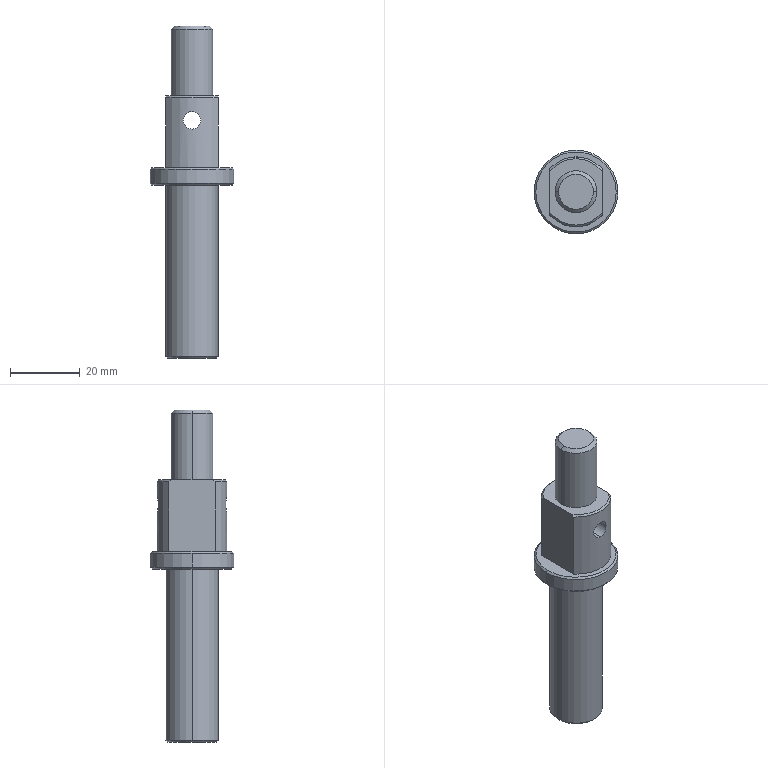Part | SolidWorks | features ICE 4, Chamfer 3, HoleWzd 2, Extrusion 1 | 1 solid | 31 faces | box 24 x 24 x 95 mm | volume 18042 mm3 | cylinder 12 | cone 12 | plane 7 | commonest cylinder face diameters 5 x4 12 x2 15 x2 20 x2 24 x2
STEP:
#1=CARTESIAN_POINT('',(0.,-10.,65.5));
#2=VERTEX_POINT('',#1);
#3=CARTESIAN_POINT('',(0.,-10.,70.5));
#4=VERTEX_POINT('',#3);
#5=CARTESIAN_POINT('',(0.,-10.,65.5));
#6=CARTESIAN_POINT('',(-0.327,-10.,65.5));
#7=CARTESIAN_POINT('',(-0.6572,-9.983,65.566));
#8=CARTESIAN_POINT('',(-1.109,-9.939,65.753));
#9=CARTESIAN_POINT('',(-1.255,-9.922,65.832));
#10=CARTESIAN_POINT('',(-1.526,-9.884,66.013));
#11=CARTESIAN_POINT('',(-1.652,-9.863,66.116));
#12=CARTESIAN_POINT('',(-1.882,-9.822,66.347));
#13=CARTESIAN_POINT('',(-1.987,-9.801,66.475));
#14=CARTESIAN_POINT('',(-2.168,-9.763,66.745));
#15=CARTESIAN_POINT('',(-2.245,-9.745,66.888));
#16=CARTESIAN_POINT('',(-2.372,-9.715,67.192));
#17=CARTESIAN_POINT('',(-2.419,-9.703,67.349));
#18=CARTESIAN_POINT('',(-2.483,-9.687,67.669));
#19=CARTESIAN_POINT('',(-2.5,-9.682,67.834));
#20=CARTESIAN_POINT('',(-2.5,-9.682,68.164));
#21=CARTESIAN_POINT('',(-2.484,-9.687,68.327));
#22=CARTESIAN_POINT('',(-2.42,-9.703,68.648));
#23=CARTESIAN_POINT('',(-2.372,-9.715,68.807));
#24=CARTESIAN_POINT('',(-2.247,-9.745,69.109));
#25=CARTESIAN_POINT('',(-2.17,-9.762,69.253));
#26=CARTESIAN_POINT('',(-1.988,-9.801,69.525));
#27=CARTESIAN_POINT('',(-1.883,-9.822,69.652));
#28=CARTESIAN_POINT('',(-1.654,-9.863,69.882));
#29=CARTESIAN_POINT('',(-1.527,-9.884,69.986));
#30=CARTESIAN_POINT('',(-1.255,-9.922,70.168));
#31=CARTESIAN_POINT('',(-1.112,-9.939,70.245));
#32=CARTESIAN_POINT('',(-0.8107,-9.968,70.371));
#33=CARTESIAN_POINT('',(-0.6515,-9.98,70.419));
#34=CARTESIAN_POINT('',(-0.3293,-9.996,70.484));
#35=CARTESIAN_POINT('',(-0.1658,-10.,70.5));
#36=CARTESIAN_POINT('',(0.,-10.,70.5));
#37=B_SPLINE_CURVE_WITH_KNOTS('',3,(#5,#6,#7,#8,#9,#10,#11,#12,#13,#14,#15,#16,#17,#18,#19,#20,#21,#22,#23,#24,#25,#26,#27,#28,#29,#30,#31,#32,#33,#34,#35,#36),.UNSPECIFIED.,.F.,.F.,(4,2,2,2,2,2,2,2,2,2,2,2,2,2,2,4),(0.007847,0.008828,0.009318,0.009809,0.0103,0.01079,0.01128,0.01177,0.01226,0.01275,0.01324,0.01373,0.01422,0.01471,0.0152,0.01569),.UNSPECIFIED.);
#38=EDGE_CURVE('',#2,#4,#37,.T.);
#39=ORIENTED_EDGE('',*,*,#38,.F.);
#40=CARTESIAN_POINT('',(0.,10.,65.5));
#41=VERTEX_POINT('',#40);
#42=CARTESIAN_POINT('',(0.,10.,65.5));
#43=DIRECTION('',(0.,1.,0.));
#44=VECTOR('',#43,1000.);
#45=LINE('',#42,#44);
#46=EDGE_CURVE('',#2,#41,#45,.T.);
#47=ORIENTED_EDGE('',*,*,#46,.T.);
#48=CARTESIAN_POINT('',(0.,10.,70.5));
#49=VERTEX_POINT('',#48);
#50=CARTESIAN_POINT('',(0.,10.,70.5));
#51=CARTESIAN_POINT('',(-0.1659,10.,70.5));
#52=CARTESIAN_POINT('',(-0.3289,9.996,70.484));
#53=CARTESIAN_POINT('',(-0.6493,9.98,70.42));
#54=CARTESIAN_POINT('',(-0.8085,9.968,70.371));
#55=CARTESIAN_POINT('',(-1.111,9.939,70.246));
#56=CARTESIAN_POINT('',(-1.254,9.922,70.169));
#57=CARTESIAN_POINT('',(-1.526,9.884,69.987));
#58=CARTESIAN_POINT('',(-1.654,9.863,69.882));
#59=CARTESIAN_POINT('',(-1.998,9.801,69.538));
#60=CARTESIAN_POINT('',(-2.184,9.759,69.26));
#61=CARTESIAN_POINT('',(-2.371,9.715,68.809));
#62=CARTESIAN_POINT('',(-2.419,9.703,68.651));
#63=CARTESIAN_POINT('',(-2.484,9.687,68.328));
#64=CARTESIAN_POINT('',(-2.5,9.682,68.165));
#65=CARTESIAN_POINT('',(-2.5,9.682,67.837));
#66=CARTESIAN_POINT('',(-2.484,9.687,67.671));
#67=CARTESIAN_POINT('',(-2.419,9.703,67.35));
#68=CARTESIAN_POINT('',(-2.372,9.715,67.193));
#69=CARTESIAN_POINT('',(-2.183,9.76,66.738));
#70=CARTESIAN_POINT('',(-1.999,9.801,66.463));
#71=CARTESIAN_POINT('',(-1.652,9.863,66.116));
#72=CARTESIAN_POINT('',(-1.526,9.884,66.013));
#73=CARTESIAN_POINT('',(-1.256,9.922,65.832));
#74=CARTESIAN_POINT('',(-1.109,9.939,65.754));
#75=CARTESIAN_POINT('',(-0.8074,9.969,65.628));
#76=CARTESIAN_POINT('',(-0.6515,9.98,65.581));
#77=CARTESIAN_POINT('',(-0.3295,9.996,65.516));
#78=CARTESIAN_POINT('',(-0.1635,10.,65.5));
#79=CARTESIAN_POINT('',(0.,10.,65.5));
#80=B_SPLINE_CURVE_WITH_KNOTS('',3,(#50,#51,#52,#53,#54,#55,#56,#57,#58,#59,#60,#61,#62,#63,#64,#65,#66,#67,#68,#69,#70,#71,#72,#73,#74,#75,#76,#77,#78,#79),.UNSPECIFIED.,.F.,.F.,(4,2,2,2,2,2,2,2,2,2,2,2,2,2,4),(0.,0.0004905,0.0009809,0.001471,0.001962,0.002943,0.003433,0.003924,0.004414,0.004905,0.005886,0.006376,0.006866,0.007357,0.007847),.UNSPECIFIED.);
#81=EDGE_CURVE('',#49,#41,#80,.T.);
#82=ORIENTED_EDGE('',*,*,#81,.F.);
#83=CARTESIAN_POINT('',(0.,10.,70.5));
#84=DIRECTION('',(0.,1.,0.));
#85=VECTOR('',#84,1000.);
#86=LINE('',#83,#85);
#87=EDGE_CURVE('',#4,#49,#86,.T.);
#88=ORIENTED_EDGE('',*,*,#87,.F.);
#89=EDGE_LOOP('',(#39,#47,#82,#88));
#90=FACE_OUTER_BOUND('',#89,.T.);
#91=CARTESIAN_POINT('',(0.,10.,68.));
#92=DIRECTION('',(0.,1.,0.));
#93=DIRECTION('',(0.,0.,1.));
#94=AXIS2_PLACEMENT_3D('',#91,#92,#93);
#95=CYLINDRICAL_SURFACE('',#94,2.5);
#96=ADVANCED_FACE('',(#90),#95,.F.);
#97=CARTESIAN_POINT('',(5.,0.,95.));
#98=VERTEX_POINT('',#97);
#99=CARTESIAN_POINT('',(-5.,0.,95.));
#100=VERTEX_POINT('',#99);
#101=CARTESIAN_POINT('',(0.,0.,95.));
#102=DIRECTION('',(0.,0.,1.));
#103=DIRECTION('',(1.,0.,0.));
#104=AXIS2_PLACEMENT_3D('',#101,#102,#103);
#105=CIRCLE('',#104,5.);
#106=EDGE_CURVE('',#98,#100,#105,.T.);
#107=ORIENTED_EDGE('',*,*,#106,.F.);
#108=CARTESIAN_POINT('',(6.,0.,94.));
#109=VERTEX_POINT('',#108);
#110=CARTESIAN_POINT('',(5.,0.,95.));
#111=DIRECTION('',(0.7071,0.,-0.7071));
#112=VECTOR('',#111,1000.);
#113=LINE('',#110,#112);
#114=EDGE_CURVE('',#98,#109,#113,.T.);
#115=ORIENTED_EDGE('',*,*,#114,.T.);
#116=CARTESIAN_POINT('',(-6.,0.,94.));
#117=VERTEX_POINT('',#116);
#118=CARTESIAN_POINT('',(0.,0.,94.));
#119=DIRECTION('',(0.,0.,-1.));
#120=DIRECTION('',(1.,0.,0.));
#121=AXIS2_PLACEMENT_3D('',#118,#119,#120);
#122=CIRCLE('',#121,6.);
#123=EDGE_CURVE('',#117,#109,#122,.T.);
#124=ORIENTED_EDGE('',*,*,#123,.F.);
#125=CARTESIAN_POINT('',(-5.,0.,95.));
#126=DIRECTION('',(-0.7071,0.,-0.7071));
#127=VECTOR('',#126,1000.);
#128=LINE('',#125,#127);
#129=EDGE_CURVE('',#100,#117,#128,.T.);
#130=ORIENTED_EDGE('',*,*,#129,.F.);
#131=EDGE_LOOP('',(#107,#115,#124,#130));
#132=FACE_OUTER_BOUND('',#131,.T.);
#133=CARTESIAN_POINT('',(0.,0.,95.));
#134=DIRECTION('',(0.,0.,-1.));
#135=DIRECTION('',(-1.,0.,0.));
#136=AXIS2_PLACEMENT_3D('',#133,#134,#135);
#137=CONICAL_SURFACE('',#136,5.,0.7854);
#138=ADVANCED_FACE('',(#132),#137,.T.);
#139=CARTESIAN_POINT('',(-7.,0.,0.));
#140=VERTEX_POINT('',#139);
#141=CARTESIAN_POINT('',(7.,0.,0.));
#142=VERTEX_POINT('',#141);
#143=CARTESIAN_POINT('',(0.,0.,0.));
#144=DIRECTION('',(0.,0.,-1.));
#145=DIRECTION('',(1.,0.,0.));
#146=AXIS2_PLACEMENT_3D('',#143,#144,#145);
#147=CIRCLE('',#146,7.);
#148=EDGE_CURVE('',#140,#142,#147,.T.);
#149=ORIENTED_EDGE('',*,*,#148,.F.);
#150=CARTESIAN_POINT('',(-7.5,0.,0.5));
#151=VERTEX_POINT('',#150);
#152=CARTESIAN_POINT('',(-7.5,0.,0.5));
#153=DIRECTION('',(-0.7071,0.,0.7071));
#154=VECTOR('',#153,1000.);
#155=LINE('',#152,#154);
#156=EDGE_CURVE('',#140,#151,#155,.T.);
#157=ORIENTED_EDGE('',*,*,#156,.T.);
#158=CARTESIAN_POINT('',(7.5,0.,0.5));
#159=VERTEX_POINT('',#158);
#160=CARTESIAN_POINT('',(0.,0.,0.5));
#161=DIRECTION('',(0.,0.,1.));
#162=DIRECTION('',(1.,0.,0.));
#163=AXIS2_PLACEMENT_3D('',#160,#161,#162);
#164=CIRCLE('',#163,7.5);
#165=EDGE_CURVE('',#159,#151,#164,.T.);
#166=ORIENTED_EDGE('',*,*,#165,.F.);
#167=CARTESIAN_POINT('',(7.5,0.,0.5));
#168=DIRECTION('',(0.7071,0.,0.7071));
#169=VECTOR('',#168,1000.);
#170=LINE('',#167,#169);
#171=EDGE_CURVE('',#142,#159,#170,.T.);
#172=ORIENTED_EDGE('',*,*,#171,.F.);
#173=EDGE_LOOP('',(#149,#157,#166,#172));
#174=FACE_OUTER_BOUND('',#173,.T.);
#175=CARTESIAN_POINT('',(0.,0.,0.5));
#176=DIRECTION('',(0.,0.,1.));
#177=DIRECTION('',(1.,0.,0.));
#178=AXIS2_PLACEMENT_3D('',#175,#176,#177);
#179=CONICAL_SURFACE('',#178,7.5,0.7854);
#180=ADVANCED_FACE('',(#174),#179,.T.);
#181=CARTESIAN_POINT('',(-11.5,0.,49.5));
#182=VERTEX_POINT('',#181);
#183=CARTESIAN_POINT('',(11.5,0.,49.5));
#184=VERTEX_POINT('',#183);
#185=CARTESIAN_POINT('',(0.,0.,49.5));
#186=DIRECTION('',(0.,0.,-1.));
#187=DIRECTION('',(1.,0.,0.));
#188=AXIS2_PLACEMENT_3D('',#185,#186,#187);
#189=CIRCLE('',#188,11.5);
#190=EDGE_CURVE('',#182,#184,#189,.T.);
#191=ORIENTED_EDGE('',*,*,#190,.F.);
#192=CARTESIAN_POINT('',(-12.,0.,50.));
#193=VERTEX_POINT('',#192);
#194=CARTESIAN_POINT('',(-12.,0.,50.));
#195=DIRECTION('',(-0.7071,0.,0.7071));
#196=VECTOR('',#195,1000.);
#197=LINE('',#194,#196);
#198=EDGE_CURVE('',#182,#193,#197,.T.);
#199=ORIENTED_EDGE('',*,*,#198,.T.);
#200=CARTESIAN_POINT('',(12.,0.,50.));
#201=VERTEX_POINT('',#200);
#202=CARTESIAN_POINT('',(0.,0.,50.));
#203=DIRECTION('',(0.,0.,1.));
#204=DIRECTION('',(1.,0.,0.));
#205=AXIS2_PLACEMENT_3D('',#202,#203,#204);
#206=CIRCLE('',#205,12.);
#207=EDGE_CURVE('',#201,#193,#206,.T.);
#208=ORIENTED_EDGE('',*,*,#207,.F.);
#209=CARTESIAN_POINT('',(12.,0.,50.));
#210=DIRECTION('',(0.7071,0.,0.7071));
#211=VECTOR('',#210,1000.);
#212=LINE('',#209,#211);
#213=EDGE_CURVE('',#184,#201,#212,.T.);
#214=ORIENTED_EDGE('',*,*,#213,.F.);
#215=EDGE_LOOP('',(#191,#199,#208,#214));
#216=FACE_OUTER_BOUND('',#215,.T.);
#217=CARTESIAN_POINT('',(0.,0.,50.));
#218=DIRECTION('',(0.,0.,1.));
#219=DIRECTION('',(1.,0.,0.));
#220=AXIS2_PLACEMENT_3D('',#217,#218,#219);
#221=CONICAL_SURFACE('',#220,12.,0.7854);
#222=ADVANCED_FACE('',(#216),#221,.T.);
#223=CARTESIAN_POINT('',(11.5,0.,54.5));
#224=VERTEX_POINT('',#223);
#225=CARTESIAN_POINT('',(-11.5,0.,54.5));
#226=VERTEX_POINT('',#225);
#227=CARTESIAN_POINT('',(0.,0.,54.5));
#228=DIRECTION('',(0.,0.,1.));
#229=DIRECTION('',(1.,0.,0.));
#230=AXIS2_PLACEMENT_3D('',#227,#228,#229);
#231=CIRCLE('',#230,11.5);
#232=EDGE_CURVE('',#224,#226,#231,.T.);
#233=ORIENTED_EDGE('',*,*,#232,.F.);
#234=CARTESIAN_POINT('',(12.,0.,54.));
#235=VERTEX_POINT('',#234);
#236=CARTESIAN_POINT('',(11.5,0.,54.5));
#237=DIRECTION('',(0.7071,0.,-0.7071));
#238=VECTOR('',#237,1000.);
#239=LINE('',#236,#238);
#240=EDGE_CURVE('',#224,#235,#239,.T.);
#241=ORIENTED_EDGE('',*,*,#240,.T.);
#242=CARTESIAN_POINT('',(-12.,0.,54.));
#243=VERTEX_POINT('',#242);
#244=CARTESIAN_POINT('',(0.,0.,54.));
#245=DIRECTION('',(0.,0.,-1.));
#246=DIRECTION('',(1.,0.,0.));
#247=AXIS2_PLACEMENT_3D('',#244,#245,#246);
#248=CIRCLE('',#247,12.);
#249=EDGE_CURVE('',#243,#235,#248,.T.);
#250=ORIENTED_EDGE('',*,*,#249,.F.);
#251=CARTESIAN_POINT('',(-11.5,0.,54.5));
#252=DIRECTION('',(-0.7071,0.,-0.7071));
#253=VECTOR('',#252,1000.);
#254=LINE('',#251,#253);
#255=EDGE_CURVE('',#226,#243,#254,.T.);
#256=ORIENTED_EDGE('',*,*,#255,.F.);
#257=EDGE_LOOP('',(#233,#241,#250,#256));
#258=FACE_OUTER_BOUND('',#257,.T.);
#259=CARTESIAN_POINT('',(0.,0.,54.5));
#260=DIRECTION('',(0.,0.,-1.));
#261=DIRECTION('',(-1.,0.,0.));
#262=AXIS2_PLACEMENT_3D('',#259,#260,#261);
#263=CONICAL_SURFACE('',#262,11.5,0.7854);
#264=ADVANCED_FACE('',(#258),#263,.T.);
#265=CARTESIAN_POINT('',(2.5,0.,15.));
#266=VERTEX_POINT('',#265);
#267=CARTESIAN_POINT('',(-2.5,0.,15.));
#268=VERTEX_POINT('',#267);
#269=CARTESIAN_POINT('',(0.,0.,15.));
#270=DIRECTION('',(0.,0.,-1.));
#271=DIRECTION('',(-1.,0.,0.));
#272=AXIS2_PLACEMENT_3D('',#269,#270,#271);
#273=CIRCLE('',#272,2.5);
#274=EDGE_CURVE('',#266,#268,#273,.T.);
#275=ORIENTED_EDGE('',*,*,#274,.F.);
#276=CARTESIAN_POINT('',(2.5,0.,0.));
#277=VERTEX_POINT('',#276);
#278=CARTESIAN_POINT('',(2.5,0.,0.));
#279=DIRECTION('',(0.,0.,-1.));
#280=VECTOR('',#279,1000.);
#281=LINE('',#278,#280);
#282=EDGE_CURVE('',#266,#277,#281,.T.);
#283=ORIENTED_EDGE('',*,*,#282,.T.);
#284=CARTESIAN_POINT('',(-2.5,0.,0.));
#285=VERTEX_POINT('',#284);
#286=CARTESIAN_POINT('',(0.,0.,0.));
#287=DIRECTION('',(0.,0.,-1.));
#288=DIRECTION('',(-1.,0.,0.));
#289=AXIS2_PLACEMENT_3D('',#286,#287,#288);
#290=CIRCLE('',#289,2.5);
#291=EDGE_CURVE('',#277,#285,#290,.T.);
#292=ORIENTED_EDGE('',*,*,#291,.T.);
#293=CARTESIAN_POINT('',(-2.5,0.,0.));
#294=DIRECTION('',(0.,0.,-1.));
#295=VECTOR('',#294,1000.);
#296=LINE('',#293,#295);
#297=EDGE_CURVE('',#268,#285,#296,.T.);
#298=ORIENTED_EDGE('',*,*,#297,.F.);
#299=EDGE_LOOP('',(#275,#283,#292,#298));
#300=FACE_OUTER_BOUND('',#299,.T.);
#301=CARTESIAN_POINT('',(0.,0.,0.));
#302=DIRECTION('',(0.,0.,-1.));
#303=DIRECTION('',(-1.,0.,0.));
#304=AXIS2_PLACEMENT_3D('',#301,#302,#303);
#305=CYLINDRICAL_SURFACE('',#304,2.5);
#306=ADVANCED_FACE('',(#300),#305,.F.);
#307=CARTESIAN_POINT('',(0.,0.,16.502));
#308=VERTEX_POINT('',#307);
#309=CARTESIAN_POINT('',(-2.5,0.,15.));
#310=DIRECTION('',(-0.8572,0.,-0.515));
#311=VECTOR('',#310,1000.);
#312=LINE('',#309,#311);
#313=EDGE_CURVE('',#308,#268,#312,.T.);
#314=ORIENTED_EDGE('',*,*,#313,.F.);
#315=CARTESIAN_POINT('',(2.5,0.,15.));
#316=DIRECTION('',(0.8572,0.,-0.515));
#317=VECTOR('',#316,1000.);
#318=LINE('',#315,#317);
#319=EDGE_CURVE('',#308,#266,#318,.T.);
#320=ORIENTED_EDGE('',*,*,#319,.T.);
#321=ORIENTED_EDGE('',*,*,#274,.T.);
#322=EDGE_LOOP('',(#314,#320,#321));
#323=FACE_OUTER_BOUND('',#322,.T.);
#324=CARTESIAN_POINT('',(0.,0.,15.));
#325=DIRECTION('',(0.,0.,-1.));
#326=DIRECTION('',(-1.,0.,0.));
#327=AXIS2_PLACEMENT_3D('',#324,#325,#326);
#328=CONICAL_SURFACE('',#327,2.5,1.03);
#329=ADVANCED_FACE('',(#323),#328,.F.);
#330=ORIENTED_EDGE('',*,*,#123,.T.);
#331=CARTESIAN_POINT('',(6.,0.,75.));
#332=VERTEX_POINT('',#331);
#333=CARTESIAN_POINT('',(6.,0.,95.));
#334=DIRECTION('',(0.,0.,-1.));
#335=VECTOR('',#334,1000.);
#336=LINE('',#333,#335);
#337=EDGE_CURVE('',#109,#332,#336,.T.);
#338=ORIENTED_EDGE('',*,*,#337,.T.);
#339=CARTESIAN_POINT('',(-6.,0.,75.));
#340=VERTEX_POINT('',#339);
#341=CARTESIAN_POINT('',(0.,0.,75.));
#342=DIRECTION('',(0.,0.,1.));
#343=DIRECTION('',(1.,0.,0.));
#344=AXIS2_PLACEMENT_3D('',#341,#342,#343);
#345=CIRCLE('',#344,6.);
#346=EDGE_CURVE('',#332,#340,#345,.T.);
#347=ORIENTED_EDGE('',*,*,#346,.T.);
#348=CARTESIAN_POINT('',(-6.,0.,95.));
#349=DIRECTION('',(0.,0.,-1.));
#350=VECTOR('',#349,1000.);
#351=LINE('',#348,#350);
#352=EDGE_CURVE('',#117,#340,#351,.T.);
#353=ORIENTED_EDGE('',*,*,#352,.F.);
#354=EDGE_LOOP('',(#330,#338,#347,#353));
#355=FACE_OUTER_BOUND('',#354,.T.);
#356=CARTESIAN_POINT('',(0.,0.,95.));
#357=DIRECTION('',(0.,0.,-1.));
#358=DIRECTION('',(-1.,0.,0.));
#359=AXIS2_PLACEMENT_3D('',#356,#357,#358);
#360=CYLINDRICAL_SURFACE('',#359,6.);
#361=ADVANCED_FACE('',(#355),#360,.T.);
#362=ORIENTED_EDGE('',*,*,#249,.T.);
#363=CARTESIAN_POINT('',(12.,0.,54.5));
#364=DIRECTION('',(0.,0.,-1.));
#365=VECTOR('',#364,1000.);
#366=LINE('',#363,#365);
#367=EDGE_CURVE('',#235,#201,#366,.T.);
#368=ORIENTED_EDGE('',*,*,#367,.T.);
#369=ORIENTED_EDGE('',*,*,#207,.T.);
#370=CARTESIAN_POINT('',(-12.,0.,54.5));
#371=DIRECTION('',(0.,0.,-1.));
#372=VECTOR('',#371,1000.);
#373=LINE('',#370,#372);
#374=EDGE_CURVE('',#243,#193,#373,.T.);
#375=ORIENTED_EDGE('',*,*,#374,.F.);
#376=EDGE_LOOP('',(#362,#368,#369,#375));
#377=FACE_OUTER_BOUND('',#376,.T.);
#378=CARTESIAN_POINT('',(0.,0.,54.5));
#379=DIRECTION('',(0.,0.,-1.));
#380=DIRECTION('',(-1.,0.,0.));
#381=AXIS2_PLACEMENT_3D('',#378,#379,#380);
#382=CYLINDRICAL_SURFACE('',#381,12.);
#383=ADVANCED_FACE('',(#377),#382,.T.);
#384=CARTESIAN_POINT('',(7.5,0.,49.5));
#385=VERTEX_POINT('',#384);
#386=CARTESIAN_POINT('',(-7.5,0.,49.5));
#387=VERTEX_POINT('',#386);
#388=CARTESIAN_POINT('',(0.,0.,49.5));
#389=DIRECTION('',(0.,0.,1.));
#390=DIRECTION('',(1.,0.,0.));
#391=AXIS2_PLACEMENT_3D('',#388,#389,#390);
#392=CIRCLE('',#391,7.5);
#393=EDGE_CURVE('',#385,#387,#392,.T.);
#394=ORIENTED_EDGE('',*,*,#393,.F.);
#395=CARTESIAN_POINT('',(7.5,0.,49.5));
#396=DIRECTION('',(0.,0.,-1.));
#397=VECTOR('',#396,1000.);
#398=LINE('',#395,#397);
#399=EDGE_CURVE('',#385,#159,#398,.T.);
#400=ORIENTED_EDGE('',*,*,#399,.T.);
#401=ORIENTED_EDGE('',*,*,#165,.T.);
#402=CARTESIAN_POINT('',(-7.5,0.,49.5));
#403=DIRECTION('',(0.,0.,-1.));
#404=VECTOR('',#403,1000.);
#405=LINE('',#402,#404);
#406=EDGE_CURVE('',#387,#151,#405,.T.);
#407=ORIENTED_EDGE('',*,*,#406,.F.);
#408=EDGE_LOOP('',(#394,#400,#401,#407));
#409=FACE_OUTER_BOUND('',#408,.T.);
#410=CARTESIAN_POINT('',(0.,0.,49.5));
#411=DIRECTION('',(0.,0.,-1.));
#412=DIRECTION('',(-1.,0.,0.));
#413=AXIS2_PLACEMENT_3D('',#410,#411,#412);
#414=CYLINDRICAL_SURFACE('',#413,7.5);
#415=ADVANCED_FACE('',(#409),#414,.T.);
#416=ORIENTED_EDGE('',*,*,#81,.T.);
#417=CARTESIAN_POINT('',(0.,10.,65.5));
#418=CARTESIAN_POINT('',(0.327,10.,65.5));
#419=CARTESIAN_POINT('',(0.6572,9.983,65.566));
#420=CARTESIAN_POINT('',(1.109,9.939,65.753));
#421=CARTESIAN_POINT('',(1.255,9.922,65.832));
#422=CARTESIAN_POINT('',(1.526,9.884,66.013));
#423=CARTESIAN_POINT('',(1.652,9.863,66.116));
#424=CARTESIAN_POINT('',(1.882,9.822,66.347));
#425=CARTESIAN_POINT('',(1.987,9.801,66.475));
#426=CARTESIAN_POINT('',(2.168,9.763,66.745));
#427=CARTESIAN_POINT('',(2.245,9.745,66.888));
#428=CARTESIAN_POINT('',(2.372,9.715,67.192));
#429=CARTESIAN_POINT('',(2.419,9.703,67.349));
#430=CARTESIAN_POINT('',(2.483,9.687,67.669));
#431=CARTESIAN_POINT('',(2.5,9.682,67.834));
#432=CARTESIAN_POINT('',(2.5,9.682,68.164));
#433=CARTESIAN_POINT('',(2.484,9.687,68.327));
#434=CARTESIAN_POINT('',(2.42,9.703,68.648));
#435=CARTESIAN_POINT('',(2.372,9.715,68.807));
#436=CARTESIAN_POINT('',(2.247,9.745,69.109));
#437=CARTESIAN_POINT('',(2.17,9.762,69.253));
#438=CARTESIAN_POINT('',(1.988,9.801,69.525));
#439=CARTESIAN_POINT('',(1.883,9.822,69.652));
#440=CARTESIAN_POINT('',(1.654,9.863,69.882));
#441=CARTESIAN_POINT('',(1.527,9.884,69.986));
#442=CARTESIAN_POINT('',(1.255,9.922,70.168));
#443=CARTESIAN_POINT('',(1.112,9.939,70.245));
#444=CARTESIAN_POINT('',(0.8107,9.968,70.371));
#445=CARTESIAN_POINT('',(0.6515,9.98,70.419));
#446=CARTESIAN_POINT('',(0.3293,9.996,70.484));
#447=CARTESIAN_POINT('',(0.1658,10.,70.5));
#448=CARTESIAN_POINT('',(0.,10.,70.5));
#449=B_SPLINE_CURVE_WITH_KNOTS('',3,(#417,#418,#419,#420,#421,#422,#423,#424,#425,#426,#427,#428,#429,#430,#431,#432,#433,#434,#435,#436,#437,#438,#439,#440,#441,#442,#443,#444,#445,#446,#447,#448),.UNSPECIFIED.,.F.,.F.,(4,2,2,2,2,2,2,2,2,2,2,2,2,2,2,4),(0.007847,0.008828,0.009318,0.009809,0.0103,0.01079,0.01128,0.01177,0.01226,0.01275,0.01324,0.01373,0.01422,0.01471,0.0152,0.01569),.UNSPECIFIED.);
#450=EDGE_CURVE('',#41,#49,#449,.T.);
#451=ORIENTED_EDGE('',*,*,#450,.T.);
#452=EDGE_LOOP('',(#416,#451));
#453=FACE_BOUND('',#452,.T.);
#454=CARTESIAN_POINT('',(-7.5,6.614,74.5));
#455=VERTEX_POINT('',#454);
#456=CARTESIAN_POINT('',(7.5,6.614,74.5));
#457=VERTEX_POINT('',#456);
#458=CARTESIAN_POINT('',(0.,0.,74.5));
#459=DIRECTION('',(0.,0.,-1.));
#460=DIRECTION('',(1.,0.,0.));
#461=AXIS2_PLACEMENT_3D('',#458,#459,#460);
#462=CIRCLE('',#461,10.);
#463=EDGE_CURVE('',#455,#457,#462,.T.);
#464=ORIENTED_EDGE('',*,*,#463,.T.);
#465=CARTESIAN_POINT('',(7.5,6.614,54.5));
#466=VERTEX_POINT('',#465);
#467=CARTESIAN_POINT('',(7.5,6.614,75.));
#468=DIRECTION('',(0.,0.,-1.));
#469=VECTOR('',#468,1000.);
#470=LINE('',#467,#469);
#471=EDGE_CURVE('',#457,#466,#470,.T.);
#472=ORIENTED_EDGE('',*,*,#471,.T.);
#473=CARTESIAN_POINT('',(-7.5,6.614,54.5));
#474=VERTEX_POINT('',#473);
#475=CARTESIAN_POINT('',(0.,0.,54.5));
#476=DIRECTION('',(0.,0.,1.));
#477=DIRECTION('',(1.,0.,0.));
#478=AXIS2_PLACEMENT_3D('',#475,#476,#477);
#479=CIRCLE('',#478,10.);
#480=EDGE_CURVE('',#466,#474,#479,.T.);
#481=ORIENTED_EDGE('',*,*,#480,.T.);
#482=CARTESIAN_POINT('',(-7.5,6.614,75.));
#483=DIRECTION('',(0.,0.,1.));
#484=VECTOR('',#483,1000.);
#485=LINE('',#482,#484);
#486=EDGE_CURVE('',#474,#455,#485,.T.);
#487=ORIENTED_EDGE('',*,*,#486,.T.);
#488=EDGE_LOOP('',(#464,#472,#481,#487));
#489=FACE_OUTER_BOUND('',#488,.T.);
#490=CARTESIAN_POINT('',(0.,0.,75.));
#491=DIRECTION('',(0.,0.,-1.));
#492=DIRECTION('',(-1.,0.,0.));
#493=AXIS2_PLACEMENT_3D('',#490,#491,#492);
#494=CYLINDRICAL_SURFACE('',#493,10.);
#495=ADVANCED_FACE('',(#453,#489),#494,.T.);
#496=CARTESIAN_POINT('',(7.5,5.831,75.));
#497=VERTEX_POINT('',#496);
#498=CARTESIAN_POINT('',(7.5,6.614,74.5));
#499=CARTESIAN_POINT('',(7.5,6.356,74.671));
#500=CARTESIAN_POINT('',(7.5,6.095,74.838));
#501=CARTESIAN_POINT('',(7.5,5.831,75.));
#502=B_SPLINE_CURVE_WITH_KNOTS('',3,(#498,#499,#500,#501),.UNSPECIFIED.,.F.,.F.,(4,4),(0.01853,0.01946),.UNSPECIFIED.);
#503=EDGE_CURVE('',#457,#497,#502,.T.);
#504=ORIENTED_EDGE('',*,*,#503,.F.);
#505=ORIENTED_EDGE('',*,*,#463,.F.);
#506=CARTESIAN_POINT('',(-7.5,5.831,75.));
#507=VERTEX_POINT('',#506);
#508=CARTESIAN_POINT('',(-7.5,5.831,75.));
#509=CARTESIAN_POINT('',(-7.5,6.095,74.838));
#510=CARTESIAN_POINT('',(-7.5,6.357,74.671));
#511=CARTESIAN_POINT('',(-7.5,6.614,74.5));
#512=B_SPLINE_CURVE_WITH_KNOTS('',3,(#508,#509,#510,#511),.UNSPECIFIED.,.F.,.F.,(4,4),(0.03186,0.03278),.UNSPECIFIED.);
#513=EDGE_CURVE('',#507,#455,#512,.T.);
#514=ORIENTED_EDGE('',*,*,#513,.F.);
#515=CARTESIAN_POINT('',(0.,0.,75.));
#516=DIRECTION('',(0.,0.,1.));
#517=DIRECTION('',(1.,0.,0.));
#518=AXIS2_PLACEMENT_3D('',#515,#516,#517);
#519=CIRCLE('',#518,9.5);
#520=EDGE_CURVE('',#497,#507,#519,.T.);
#521=ORIENTED_EDGE('',*,*,#520,.F.);
#522=EDGE_LOOP('',(#504,#505,#514,#521));
#523=FACE_OUTER_BOUND('',#522,.T.);
#524=CARTESIAN_POINT('',(0.,0.,75.));
#525=DIRECTION('',(0.,0.,-1.));
#526=DIRECTION('',(-1.,0.,0.));
#527=AXIS2_PLACEMENT_3D('',#524,#525,#526);
#528=CONICAL_SURFACE('',#527,9.5,0.7854);
#529=ADVANCED_FACE('',(#523),#528,.T.);
#530=CARTESIAN_POINT('',(7.5,-5.831,75.));
#531=VERTEX_POINT('',#530);
#532=CARTESIAN_POINT('',(7.5,0.,75.));
#533=DIRECTION('',(0.,-1.,0.));
#534=VECTOR('',#533,1000.);
#535=LINE('',#532,#534);
#536=EDGE_CURVE('',#497,#531,#535,.T.);
#537=ORIENTED_EDGE('',*,*,#536,.F.);
#538=ORIENTED_EDGE('',*,*,#520,.T.);
#539=CARTESIAN_POINT('',(-7.5,-5.831,75.));
#540=VERTEX_POINT('',#539);
#541=CARTESIAN_POINT('',(-7.5,0.,75.));
#542=DIRECTION('',(0.,1.,0.));
#543=VECTOR('',#542,1000.);
#544=LINE('',#541,#543);
#545=EDGE_CURVE('',#540,#507,#544,.T.);
#546=ORIENTED_EDGE('',*,*,#545,.F.);
#547=CARTESIAN_POINT('',(0.,0.,75.));
#548=DIRECTION('',(0.,0.,1.));
#549=DIRECTION('',(1.,0.,0.));
#550=AXIS2_PLACEMENT_3D('',#547,#548,#549);
#551=CIRCLE('',#550,9.5);
#552=EDGE_CURVE('',#540,#531,#551,.T.);
#553=ORIENTED_EDGE('',*,*,#552,.T.);
#554=EDGE_LOOP('',(#537,#538,#546,#553));
#555=FACE_OUTER_BOUND('',#554,.T.);
#556=CARTESIAN_POINT('',(0.,0.,75.));
#557=DIRECTION('',(0.,0.,1.));
#558=DIRECTION('',(1.,0.,0.));
#559=AXIS2_PLACEMENT_3D('',#556,#557,#558);
#560=CIRCLE('',#559,6.);
#561=EDGE_CURVE('',#340,#332,#560,.T.);
#562=ORIENTED_EDGE('',*,*,#561,.F.);
#563=ORIENTED_EDGE('',*,*,#346,.F.);
#564=EDGE_LOOP('',(#562,#563));
#565=FACE_BOUND('',#564,.T.);
#566=CARTESIAN_POINT('',(0.,0.,75.));
#567=DIRECTION('',(0.,0.,1.));
#568=DIRECTION('',(1.,0.,0.));
#569=AXIS2_PLACEMENT_3D('',#566,#567,#568);
#570=PLANE('',#569);
#571=ADVANCED_FACE('',(#555,#565),#570,.T.);
#572=ORIENTED_EDGE('',*,*,#480,.F.);
#573=CARTESIAN_POINT('',(7.5,-6.614,54.5));
#574=VERTEX_POINT('',#573);
#575=CARTESIAN_POINT('',(7.5,-52.,54.5));
#576=DIRECTION('',(0.,1.,0.));
#577=VECTOR('',#576,1000.);
#578=LINE('',#575,#577);
#579=EDGE_CURVE('',#574,#466,#578,.T.);
#580=ORIENTED_EDGE('',*,*,#579,.F.);
#581=CARTESIAN_POINT('',(-7.5,-6.614,54.5));
#582=VERTEX_POINT('',#581);
#583=CARTESIAN_POINT('',(0.,0.,54.5));
#584=DIRECTION('',(0.,0.,1.));
#585=DIRECTION('',(1.,0.,0.));
#586=AXIS2_PLACEMENT_3D('',#583,#584,#585);
#587=CIRCLE('',#586,10.);
#588=EDGE_CURVE('',#582,#574,#587,.T.);
#589=ORIENTED_EDGE('',*,*,#588,.F.);
#590=CARTESIAN_POINT('',(-7.5,-52.,54.5));
#591=DIRECTION('',(0.,1.,0.));
#592=VECTOR('',#591,1000.);
#593=LINE('',#590,#592);
#594=EDGE_CURVE('',#582,#474,#593,.T.);
#595=ORIENTED_EDGE('',*,*,#594,.T.);
#596=EDGE_LOOP('',(#572,#580,#589,#595));
#597=FACE_BOUND('',#596,.T.);
#598=CARTESIAN_POINT('',(0.,0.,54.5));
#599=DIRECTION('',(0.,0.,1.));
#600=DIRECTION('',(1.,0.,0.));
#601=AXIS2_PLACEMENT_3D('',#598,#599,#600);
#602=CIRCLE('',#601,11.5);
#603=EDGE_CURVE('',#226,#224,#602,.T.);
#604=ORIENTED_EDGE('',*,*,#603,.T.);
#605=ORIENTED_EDGE('',*,*,#232,.T.);
#606=EDGE_LOOP('',(#604,#605));
#607=FACE_OUTER_BOUND('',#606,.T.);
#608=CARTESIAN_POINT('',(0.,0.,54.5));
#609=DIRECTION('',(0.,0.,1.));
#610=DIRECTION('',(1.,0.,0.));
#611=AXIS2_PLACEMENT_3D('',#608,#609,#610);
#612=PLANE('',#611);
#613=ADVANCED_FACE('',(#597,#607),#612,.T.);
#614=ORIENTED_EDGE('',*,*,#399,.F.);
#615=CARTESIAN_POINT('',(0.,0.,49.5));
#616=DIRECTION('',(0.,0.,1.));
#617=DIRECTION('',(1.,0.,0.));
#618=AXIS2_PLACEMENT_3D('',#615,#616,#617);
#619=CIRCLE('',#618,7.5);
#620=EDGE_CURVE('',#387,#385,#619,.T.);
#621=ORIENTED_EDGE('',*,*,#620,.F.);
#622=ORIENTED_EDGE('',*,*,#406,.T.);
#623=CARTESIAN_POINT('',(0.,0.,0.5));
#624=DIRECTION('',(0.,0.,1.));
#625=DIRECTION('',(1.,0.,0.));
#626=AXIS2_PLACEMENT_3D('',#623,#624,#625);
#627=CIRCLE('',#626,7.5);
#628=EDGE_CURVE('',#151,#159,#627,.T.);
#629=ORIENTED_EDGE('',*,*,#628,.T.);
#630=EDGE_LOOP('',(#614,#621,#622,#629));
#631=FACE_OUTER_BOUND('',#630,.T.);
#632=CARTESIAN_POINT('',(0.,0.,49.5));
#633=DIRECTION('',(0.,0.,-1.));
#634=DIRECTION('',(-1.,0.,0.));
#635=AXIS2_PLACEMENT_3D('',#632,#633,#634);
#636=CYLINDRICAL_SURFACE('',#635,7.5);
#637=ADVANCED_FACE('',(#631),#636,.T.);
#638=CARTESIAN_POINT('',(0.,0.,0.));
#639=DIRECTION('',(0.,0.,-1.));
#640=DIRECTION('',(1.,0.,0.));
#641=AXIS2_PLACEMENT_3D('',#638,#639,#640);
#642=CIRCLE('',#641,7.);
#643=EDGE_CURVE('',#142,#140,#642,.T.);
#644=ORIENTED_EDGE('',*,*,#643,.T.);
#645=ORIENTED_EDGE('',*,*,#148,.T.);
#646=EDGE_LOOP('',(#644,#645));
#647=FACE_OUTER_BOUND('',#646,.T.);
#648=CARTESIAN_POINT('',(0.,0.,0.));
#649=DIRECTION('',(0.,0.,-1.));
#650=DIRECTION('',(-1.,0.,0.));
#651=AXIS2_PLACEMENT_3D('',#648,#649,#650);
#652=CIRCLE('',#651,2.5);
#653=EDGE_CURVE('',#285,#277,#652,.T.);
#654=ORIENTED_EDGE('',*,*,#653,.F.);
#655=ORIENTED_EDGE('',*,*,#291,.F.);
#656=EDGE_LOOP('',(#654,#655));
#657=FACE_BOUND('',#656,.T.);
#658=CARTESIAN_POINT('',(0.,0.,0.));
#659=DIRECTION('',(0.,0.,1.));
#660=DIRECTION('',(1.,0.,0.));
#661=AXIS2_PLACEMENT_3D('',#658,#659,#660);
#662=PLANE('',#661);
#663=ADVANCED_FACE('',(#647,#657),#662,.F.);
#664=CARTESIAN_POINT('',(0.,0.,49.5));
#665=DIRECTION('',(0.,0.,-1.));
#666=DIRECTION('',(1.,0.,0.));
#667=AXIS2_PLACEMENT_3D('',#664,#665,#666);
#668=CIRCLE('',#667,11.5);
#669=EDGE_CURVE('',#184,#182,#668,.T.);
#670=ORIENTED_EDGE('',*,*,#669,.T.);
#671=ORIENTED_EDGE('',*,*,#190,.T.);
#672=EDGE_LOOP('',(#670,#671));
#673=FACE_OUTER_BOUND('',#672,.T.);
#674=ORIENTED_EDGE('',*,*,#620,.T.);
#675=ORIENTED_EDGE('',*,*,#393,.T.);
#676=EDGE_LOOP('',(#674,#675));
#677=FACE_BOUND('',#676,.T.);
#678=CARTESIAN_POINT('',(0.,0.,49.5));
#679=DIRECTION('',(0.,0.,1.));
#680=DIRECTION('',(1.,0.,0.));
#681=AXIS2_PLACEMENT_3D('',#678,#679,#680);
#682=PLANE('',#681);
#683=ADVANCED_FACE('',(#673,#677),#682,.F.);
#684=ORIENTED_EDGE('',*,*,#367,.F.);
#685=CARTESIAN_POINT('',(0.,0.,54.));
#686=DIRECTION('',(0.,0.,-1.));
#687=DIRECTION('',(1.,0.,0.));
#688=AXIS2_PLACEMENT_3D('',#685,#686,#687);
#689=CIRCLE('',#688,12.);
#690=EDGE_CURVE('',#235,#243,#689,.T.);
#691=ORIENTED_EDGE('',*,*,#690,.T.);
#692=ORIENTED_EDGE('',*,*,#374,.T.);
#693=CARTESIAN_POINT('',(0.,0.,50.));
#694=DIRECTION('',(0.,0.,1.));
#695=DIRECTION('',(1.,0.,0.));
#696=AXIS2_PLACEMENT_3D('',#693,#694,#695);
#697=CIRCLE('',#696,12.);
#698=EDGE_CURVE('',#193,#201,#697,.T.);
#699=ORIENTED_EDGE('',*,*,#698,.T.);
#700=EDGE_LOOP('',(#684,#691,#692,#699));
#701=FACE_OUTER_BOUND('',#700,.T.);
#702=CARTESIAN_POINT('',(0.,0.,54.5));
#703=DIRECTION('',(0.,0.,-1.));
#704=DIRECTION('',(-1.,0.,0.));
#705=AXIS2_PLACEMENT_3D('',#702,#703,#704);
#706=CYLINDRICAL_SURFACE('',#705,12.);
#707=ADVANCED_FACE('',(#701),#706,.T.);
#708=CARTESIAN_POINT('',(0.,-10.,70.5));
#709=CARTESIAN_POINT('',(0.1659,-10.,70.5));
#710=CARTESIAN_POINT('',(0.3289,-9.996,70.484));
#711=CARTESIAN_POINT('',(0.6493,-9.98,70.42));
#712=CARTESIAN_POINT('',(0.8085,-9.968,70.371));
#713=CARTESIAN_POINT('',(1.111,-9.939,70.246));
#714=CARTESIAN_POINT('',(1.254,-9.922,70.169));
#715=CARTESIAN_POINT('',(1.526,-9.884,69.987));
#716=CARTESIAN_POINT('',(1.654,-9.863,69.882));
#717=CARTESIAN_POINT('',(1.998,-9.801,69.538));
#718=CARTESIAN_POINT('',(2.184,-9.759,69.26));
#719=CARTESIAN_POINT('',(2.371,-9.715,68.809));
#720=CARTESIAN_POINT('',(2.419,-9.703,68.651));
#721=CARTESIAN_POINT('',(2.484,-9.687,68.328));
#722=CARTESIAN_POINT('',(2.5,-9.682,68.165));
#723=CARTESIAN_POINT('',(2.5,-9.682,67.837));
#724=CARTESIAN_POINT('',(2.484,-9.687,67.671));
#725=CARTESIAN_POINT('',(2.419,-9.703,67.35));
#726=CARTESIAN_POINT('',(2.372,-9.715,67.193));
#727=CARTESIAN_POINT('',(2.183,-9.76,66.738));
#728=CARTESIAN_POINT('',(1.999,-9.801,66.463));
#729=CARTESIAN_POINT('',(1.652,-9.863,66.116));
#730=CARTESIAN_POINT('',(1.526,-9.884,66.013));
#731=CARTESIAN_POINT('',(1.256,-9.922,65.832));
#732=CARTESIAN_POINT('',(1.109,-9.939,65.754));
#733=CARTESIAN_POINT('',(0.8074,-9.969,65.628));
#734=CARTESIAN_POINT('',(0.6515,-9.98,65.581));
#735=CARTESIAN_POINT('',(0.3295,-9.996,65.516));
#736=CARTESIAN_POINT('',(0.1635,-10.,65.5));
#737=CARTESIAN_POINT('',(0.,-10.,65.5));
#738=B_SPLINE_CURVE_WITH_KNOTS('',3,(#708,#709,#710,#711,#712,#713,#714,#715,#716,#717,#718,#719,#720,#721,#722,#723,#724,#725,#726,#727,#728,#729,#730,#731,#732,#733,#734,#735,#736,#737),.UNSPECIFIED.,.F.,.F.,(4,2,2,2,2,2,2,2,2,2,2,2,2,2,4),(0.,0.0004905,0.0009809,0.001471,0.001962,0.002943,0.003433,0.003924,0.004414,0.004905,0.005886,0.006376,0.006866,0.007357,0.007847),.UNSPECIFIED.);
#739=EDGE_CURVE('',#4,#2,#738,.T.);
#740=ORIENTED_EDGE('',*,*,#739,.T.);
#741=ORIENTED_EDGE('',*,*,#38,.T.);
#742=EDGE_LOOP('',(#740,#741));
#743=FACE_BOUND('',#742,.T.);
#744=ORIENTED_EDGE('',*,*,#588,.T.);
#745=CARTESIAN_POINT('',(7.5,-6.614,74.5));
#746=VERTEX_POINT('',#745);
#747=CARTESIAN_POINT('',(7.5,-6.614,75.));
#748=DIRECTION('',(0.,0.,1.));
#749=VECTOR('',#748,1000.);
#750=LINE('',#747,#749);
#751=EDGE_CURVE('',#574,#746,#750,.T.);
#752=ORIENTED_EDGE('',*,*,#751,.T.);
#753=CARTESIAN_POINT('',(-7.5,-6.614,74.5));
#754=VERTEX_POINT('',#753);
#755=CARTESIAN_POINT('',(0.,0.,74.5));
#756=DIRECTION('',(0.,0.,-1.));
#757=DIRECTION('',(1.,0.,0.));
#758=AXIS2_PLACEMENT_3D('',#755,#756,#757);
#759=CIRCLE('',#758,10.);
#760=EDGE_CURVE('',#746,#754,#759,.T.);
#761=ORIENTED_EDGE('',*,*,#760,.T.);
#762=CARTESIAN_POINT('',(-7.5,-6.614,75.));
#763=DIRECTION('',(0.,0.,-1.));
#764=VECTOR('',#763,1000.);
#765=LINE('',#762,#764);
#766=EDGE_CURVE('',#754,#582,#765,.T.);
#767=ORIENTED_EDGE('',*,*,#766,.T.);
#768=EDGE_LOOP('',(#744,#752,#761,#767));
#769=FACE_OUTER_BOUND('',#768,.T.);
#770=CARTESIAN_POINT('',(0.,0.,75.));
#771=DIRECTION('',(0.,0.,-1.));
#772=DIRECTION('',(-1.,0.,0.));
#773=AXIS2_PLACEMENT_3D('',#770,#771,#772);
#774=CYLINDRICAL_SURFACE('',#773,10.);
#775=ADVANCED_FACE('',(#743,#769),#774,.T.);
#776=ORIENTED_EDGE('',*,*,#337,.F.);
#777=CARTESIAN_POINT('',(0.,0.,94.));
#778=DIRECTION('',(0.,0.,-1.));
#779=DIRECTION('',(1.,0.,0.));
#780=AXIS2_PLACEMENT_3D('',#777,#778,#779);
#781=CIRCLE('',#780,6.);
#782=EDGE_CURVE('',#109,#117,#781,.T.);
#783=ORIENTED_EDGE('',*,*,#782,.T.);
#784=ORIENTED_EDGE('',*,*,#352,.T.);
#785=ORIENTED_EDGE('',*,*,#561,.T.);
#786=EDGE_LOOP('',(#776,#783,#784,#785));
#787=FACE_OUTER_BOUND('',#786,.T.);
#788=CARTESIAN_POINT('',(0.,0.,95.));
#789=DIRECTION('',(0.,0.,-1.));
#790=DIRECTION('',(-1.,0.,0.));
#791=AXIS2_PLACEMENT_3D('',#788,#789,#790);
#792=CYLINDRICAL_SURFACE('',#791,6.);
#793=ADVANCED_FACE('',(#787),#792,.T.);
#794=CARTESIAN_POINT('',(0.,0.,95.));
#795=DIRECTION('',(0.,0.,1.));
#796=DIRECTION('',(1.,0.,0.));
#797=AXIS2_PLACEMENT_3D('',#794,#795,#796);
#798=CIRCLE('',#797,5.);
#799=EDGE_CURVE('',#100,#98,#798,.T.);
#800=ORIENTED_EDGE('',*,*,#799,.T.);
#801=ORIENTED_EDGE('',*,*,#106,.T.);
#802=EDGE_LOOP('',(#800,#801));
#803=FACE_OUTER_BOUND('',#802,.T.);
#804=CARTESIAN_POINT('',(0.,0.,95.));
#805=DIRECTION('',(0.,0.,1.));
#806=DIRECTION('',(1.,0.,0.));
#807=AXIS2_PLACEMENT_3D('',#804,#805,#806);
#808=PLANE('',#807);
#809=ADVANCED_FACE('',(#803),#808,.T.);
#810=ORIENTED_EDGE('',*,*,#319,.F.);
#811=ORIENTED_EDGE('',*,*,#313,.T.);
#812=CARTESIAN_POINT('',(0.,0.,15.));
#813=DIRECTION('',(0.,0.,-1.));
#814=DIRECTION('',(-1.,0.,0.));
#815=AXIS2_PLACEMENT_3D('',#812,#813,#814);
#816=CIRCLE('',#815,2.5);
#817=EDGE_CURVE('',#268,#266,#816,.T.);
#818=ORIENTED_EDGE('',*,*,#817,.T.);
#819=EDGE_LOOP('',(#810,#811,#818));
#820=FACE_OUTER_BOUND('',#819,.T.);
#821=CARTESIAN_POINT('',(0.,0.,15.));
#822=DIRECTION('',(0.,0.,-1.));
#823=DIRECTION('',(-1.,0.,0.));
#824=AXIS2_PLACEMENT_3D('',#821,#822,#823);
#825=CONICAL_SURFACE('',#824,2.5,1.03);
#826=ADVANCED_FACE('',(#820),#825,.F.);
#827=ORIENTED_EDGE('',*,*,#282,.F.);
#828=ORIENTED_EDGE('',*,*,#817,.F.);
#829=ORIENTED_EDGE('',*,*,#297,.T.);
#830=ORIENTED_EDGE('',*,*,#653,.T.);
#831=EDGE_LOOP('',(#827,#828,#829,#830));
#832=FACE_OUTER_BOUND('',#831,.T.);
#833=CARTESIAN_POINT('',(0.,0.,0.));
#834=DIRECTION('',(0.,0.,-1.));
#835=DIRECTION('',(-1.,0.,0.));
#836=AXIS2_PLACEMENT_3D('',#833,#834,#835);
#837=CYLINDRICAL_SURFACE('',#836,2.5);
#838=ADVANCED_FACE('',(#832),#837,.F.);
#839=ORIENTED_EDGE('',*,*,#240,.F.);
#840=ORIENTED_EDGE('',*,*,#603,.F.);
#841=ORIENTED_EDGE('',*,*,#255,.T.);
#842=ORIENTED_EDGE('',*,*,#690,.F.);
#843=EDGE_LOOP('',(#839,#840,#841,#842));
#844=FACE_OUTER_BOUND('',#843,.T.);
#845=CARTESIAN_POINT('',(0.,0.,54.5));
#846=DIRECTION('',(0.,0.,-1.));
#847=DIRECTION('',(-1.,0.,0.));
#848=AXIS2_PLACEMENT_3D('',#845,#846,#847);
#849=CONICAL_SURFACE('',#848,11.5,0.7854);
#850=ADVANCED_FACE('',(#844),#849,.T.);
#851=ORIENTED_EDGE('',*,*,#198,.F.);
#852=ORIENTED_EDGE('',*,*,#669,.F.);
#853=ORIENTED_EDGE('',*,*,#213,.T.);
#854=ORIENTED_EDGE('',*,*,#698,.F.);
#855=EDGE_LOOP('',(#851,#852,#853,#854));
#856=FACE_OUTER_BOUND('',#855,.T.);
#857=CARTESIAN_POINT('',(0.,0.,50.));
#858=DIRECTION('',(0.,0.,1.));
#859=DIRECTION('',(1.,0.,0.));
#860=AXIS2_PLACEMENT_3D('',#857,#858,#859);
#861=CONICAL_SURFACE('',#860,12.,0.7854);
#862=ADVANCED_FACE('',(#856),#861,.T.);
#863=ORIENTED_EDGE('',*,*,#156,.F.);
#864=ORIENTED_EDGE('',*,*,#643,.F.);
#865=ORIENTED_EDGE('',*,*,#171,.T.);
#866=ORIENTED_EDGE('',*,*,#628,.F.);
#867=EDGE_LOOP('',(#863,#864,#865,#866));
#868=FACE_OUTER_BOUND('',#867,.T.);
#869=CARTESIAN_POINT('',(0.,0.,0.5));
#870=DIRECTION('',(0.,0.,1.));
#871=DIRECTION('',(1.,0.,0.));
#872=AXIS2_PLACEMENT_3D('',#869,#870,#871);
#873=CONICAL_SURFACE('',#872,7.5,0.7854);
#874=ADVANCED_FACE('',(#868),#873,.T.);
#875=ORIENTED_EDGE('',*,*,#114,.F.);
#876=ORIENTED_EDGE('',*,*,#799,.F.);
#877=ORIENTED_EDGE('',*,*,#129,.T.);
#878=ORIENTED_EDGE('',*,*,#782,.F.);
#879=EDGE_LOOP('',(#875,#876,#877,#878));
#880=FACE_OUTER_BOUND('',#879,.T.);
#881=CARTESIAN_POINT('',(0.,0.,95.));
#882=DIRECTION('',(0.,0.,-1.));
#883=DIRECTION('',(-1.,0.,0.));
#884=AXIS2_PLACEMENT_3D('',#881,#882,#883);
#885=CONICAL_SURFACE('',#884,5.,0.7854);
#886=ADVANCED_FACE('',(#880),#885,.T.);
#887=CARTESIAN_POINT('',(7.5,-5.831,75.));
#888=CARTESIAN_POINT('',(7.5,-6.095,74.838));
#889=CARTESIAN_POINT('',(7.5,-6.357,74.671));
#890=CARTESIAN_POINT('',(7.5,-6.614,74.5));
#891=B_SPLINE_CURVE_WITH_KNOTS('',3,(#887,#888,#889,#890),.UNSPECIFIED.,.F.,.F.,(4,4),(0.03186,0.03278),.UNSPECIFIED.);
#892=EDGE_CURVE('',#531,#746,#891,.T.);
#893=ORIENTED_EDGE('',*,*,#892,.F.);
#894=ORIENTED_EDGE('',*,*,#552,.F.);
#895=CARTESIAN_POINT('',(-7.5,-6.614,74.5));
#896=CARTESIAN_POINT('',(-7.5,-6.356,74.671));
#897=CARTESIAN_POINT('',(-7.5,-6.095,74.838));
#898=CARTESIAN_POINT('',(-7.5,-5.831,75.));
#899=B_SPLINE_CURVE_WITH_KNOTS('',3,(#895,#896,#897,#898),.UNSPECIFIED.,.F.,.F.,(4,4),(0.01853,0.01946),.UNSPECIFIED.);
#900=EDGE_CURVE('',#754,#540,#899,.T.);
#901=ORIENTED_EDGE('',*,*,#900,.F.);
#902=ORIENTED_EDGE('',*,*,#760,.F.);
#903=EDGE_LOOP('',(#893,#894,#901,#902));
#904=FACE_OUTER_BOUND('',#903,.T.);
#905=CARTESIAN_POINT('',(0.,0.,75.));
#906=DIRECTION('',(0.,0.,-1.));
#907=DIRECTION('',(-1.,0.,0.));
#908=AXIS2_PLACEMENT_3D('',#905,#906,#907);
#909=CONICAL_SURFACE('',#908,9.5,0.7854);
#910=ADVANCED_FACE('',(#904),#909,.T.);
#911=ORIENTED_EDGE('',*,*,#900,.T.);
#912=ORIENTED_EDGE('',*,*,#545,.T.);
#913=ORIENTED_EDGE('',*,*,#513,.T.);
#914=ORIENTED_EDGE('',*,*,#486,.F.);
#915=ORIENTED_EDGE('',*,*,#594,.F.);
#916=ORIENTED_EDGE('',*,*,#766,.F.);
#917=EDGE_LOOP('',(#911,#912,#913,#914,#915,#916));
#918=FACE_OUTER_BOUND('',#917,.T.);
#919=CARTESIAN_POINT('',(-7.5,-52.,54.5));
#920=DIRECTION('',(1.,0.,0.));
#921=DIRECTION('',(0.,0.,-1.));
#922=AXIS2_PLACEMENT_3D('',#919,#920,#921);
#923=PLANE('',#922);
#924=ADVANCED_FACE('',(#918),#923,.F.);
#925=ORIENTED_EDGE('',*,*,#503,.T.);
#926=ORIENTED_EDGE('',*,*,#536,.T.);
#927=ORIENTED_EDGE('',*,*,#892,.T.);
#928=ORIENTED_EDGE('',*,*,#751,.F.);
#929=ORIENTED_EDGE('',*,*,#579,.T.);
#930=ORIENTED_EDGE('',*,*,#471,.F.);
#931=EDGE_LOOP('',(#925,#926,#927,#928,#929,#930));
#932=FACE_OUTER_BOUND('',#931,.T.);
#933=CARTESIAN_POINT('',(7.5,-52.,54.5));
#934=DIRECTION('',(-1.,0.,0.));
#935=DIRECTION('',(0.,0.,1.));
#936=AXIS2_PLACEMENT_3D('',#933,#934,#935);
#937=PLANE('',#936);
#938=ADVANCED_FACE('',(#932),#937,.F.);
#939=ORIENTED_EDGE('',*,*,#46,.F.);
#940=ORIENTED_EDGE('',*,*,#739,.F.);
#941=ORIENTED_EDGE('',*,*,#87,.T.);
#942=ORIENTED_EDGE('',*,*,#450,.F.);
#943=EDGE_LOOP('',(#939,#940,#941,#942));
#944=FACE_OUTER_BOUND('',#943,.T.);
#945=CARTESIAN_POINT('',(0.,10.,68.));
#946=DIRECTION('',(0.,1.,0.));
#947=DIRECTION('',(0.,0.,1.));
#948=AXIS2_PLACEMENT_3D('',#945,#946,#947);
#949=CYLINDRICAL_SURFACE('',#948,2.5);
#950=ADVANCED_FACE('',(#944),#949,.F.);
#951=CLOSED_SHELL('',(#96,#138,#180,#222,#264,#306,#329,#361,#383,#415,#495,#529,#571,#613,#637,#663,#683,#707,#775,#793,#809,#826,#838,#850,#862,#874,#886,#910,#924,#938,#950));
#952=MANIFOLD_SOLID_BREP('',#951);
#953=CARTESIAN_POINT('',(0.,0.,0.));
#954=DIRECTION('',(0.,0.,1.));
#955=DIRECTION('',(1.,0.,0.));
#956=AXIS2_PLACEMENT_3D('',#953,#954,#955);
#957=(LENGTH_UNIT()NAMED_UNIT(*)SI_UNIT(.MILLI.,.METRE.));
#958=UNCERTAINTY_MEASURE_WITH_UNIT(LENGTH_MEASURE(0.00001),#957,'','');
#959=(NAMED_UNIT(*)PLANE_ANGLE_UNIT()SI_UNIT($,.RADIAN.));
#960=(NAMED_UNIT(*)SI_UNIT($,.STERADIAN.)SOLID_ANGLE_UNIT());
#961=(GEOMETRIC_REPRESENTATION_CONTEXT(3)GLOBAL_UNCERTAINTY_ASSIGNED_CONTEXT((#958))GLOBAL_UNIT_ASSIGNED_CONTEXT((#957,#959,#960))REPRESENTATION_CONTEXT('',''));
#962=ADVANCED_BREP_SHAPE_REPRESENTATION('',(#952,#956),#961);